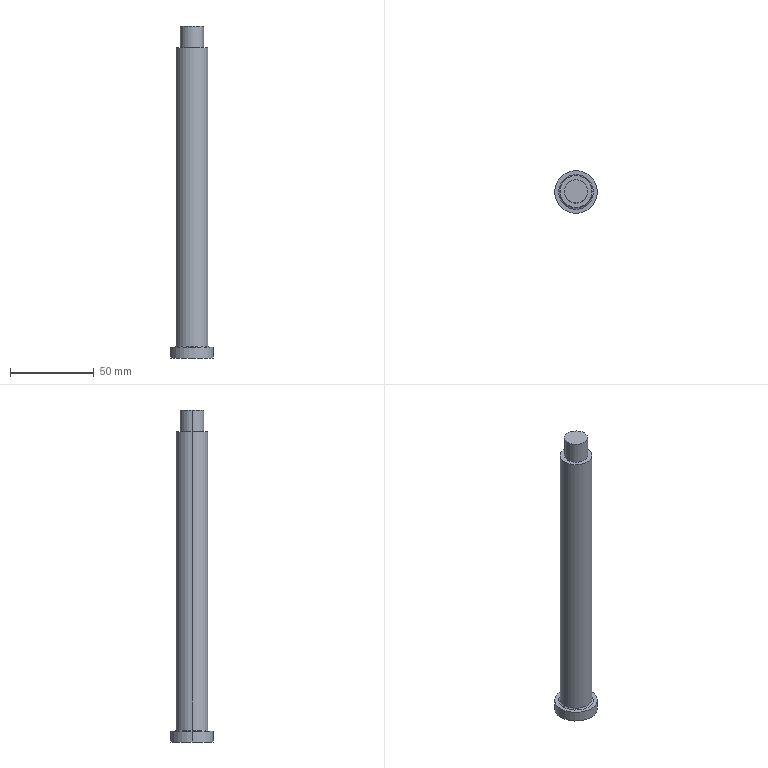Part | STEP file | 4-20.sldasm-Part-374 | 1 solid | 12 faces | box 25.4 x 25.4 x 198 mm | volume 56107 mm3 | cylinder 6 | plane 4 | torus 2 | commonest cylinder face diameters 13.862 x2 19.05 x2 25.4 x2
STEP:
#1=CARTESIAN_POINT('',(4.931,227.,93.));
#2=VERTEX_POINT('',#1);
#3=CARTESIAN_POINT('',(-8.931,227.,93.));
#4=VERTEX_POINT('',#3);
#5=CARTESIAN_POINT('',(-2.,227.,93.));
#6=DIRECTION('',(0.,0.,1.));
#7=DIRECTION('',(-1.,0.,0.));
#8=AXIS2_PLACEMENT_3D('',#5,#6,#7);
#9=CIRCLE('',#8,6.931);
#10=EDGE_CURVE('',#2,#4,#9,.T.);
#11=ORIENTED_EDGE('',*,*,#10,.F.);
#12=CARTESIAN_POINT('',(4.931,227.,80.));
#13=VERTEX_POINT('',#12);
#14=CARTESIAN_POINT('',(4.931,227.,62.4));
#15=DIRECTION('',(0.,0.,-1.));
#16=VECTOR('',#15,1000.);
#17=LINE('',#14,#16);
#18=EDGE_CURVE('',#2,#13,#17,.T.);
#19=ORIENTED_EDGE('',*,*,#18,.T.);
#20=CARTESIAN_POINT('',(-8.931,227.,80.));
#21=VERTEX_POINT('',#20);
#22=CARTESIAN_POINT('',(-2.,227.,80.));
#23=DIRECTION('',(0.,0.,1.));
#24=DIRECTION('',(1.,0.,0.));
#25=AXIS2_PLACEMENT_3D('',#22,#23,#24);
#26=CIRCLE('',#25,6.931);
#27=EDGE_CURVE('',#13,#21,#26,.T.);
#28=ORIENTED_EDGE('',*,*,#27,.T.);
#29=CARTESIAN_POINT('',(-8.931,227.,62.4));
#30=DIRECTION('',(0.,0.,-1.));
#31=VECTOR('',#30,1000.);
#32=LINE('',#29,#31);
#33=EDGE_CURVE('',#4,#21,#32,.T.);
#34=ORIENTED_EDGE('',*,*,#33,.F.);
#35=EDGE_LOOP('',(#11,#19,#28,#34));
#36=FACE_OUTER_BOUND('',#35,.T.);
#37=CARTESIAN_POINT('',(-2.,227.,62.4));
#38=DIRECTION('',(0.,0.,-1.));
#39=DIRECTION('',(-1.,0.,0.));
#40=AXIS2_PLACEMENT_3D('',#37,#38,#39);
#41=CYLINDRICAL_SURFACE('',#40,6.931);
#42=ADVANCED_FACE('',(#36),#41,.T.);
#43=CARTESIAN_POINT('',(-12.319,227.,-98.65));
#44=VERTEX_POINT('',#43);
#45=CARTESIAN_POINT('',(8.319,227.,-98.65));
#46=VERTEX_POINT('',#45);
#47=CARTESIAN_POINT('',(-2.,227.,-98.65));
#48=DIRECTION('',(0.,0.,1.));
#49=DIRECTION('',(0.,-1.,0.));
#50=AXIS2_PLACEMENT_3D('',#47,#48,#49);
#51=CIRCLE('',#50,10.319);
#52=EDGE_CURVE('',#44,#46,#51,.T.);
#53=ORIENTED_EDGE('',*,*,#52,.T.);
#54=CARTESIAN_POINT('',(7.525,227.,-97.856));
#55=VERTEX_POINT('',#54);
#56=CARTESIAN_POINT('',(8.319,227.,-97.856));
#57=DIRECTION('',(0.,1.,0.));
#58=DIRECTION('',(-1.,0.,0.));
#59=AXIS2_PLACEMENT_3D('',#56,#57,#58);
#60=CIRCLE('',#59,0.7938);
#61=EDGE_CURVE('',#46,#55,#60,.T.);
#62=ORIENTED_EDGE('',*,*,#61,.T.);
#63=CARTESIAN_POINT('',(-11.525,227.,-97.856));
#64=VERTEX_POINT('',#63);
#65=CARTESIAN_POINT('',(-2.,227.,-97.856));
#66=DIRECTION('',(0.,0.,1.));
#67=DIRECTION('',(0.,-1.,0.));
#68=AXIS2_PLACEMENT_3D('',#65,#66,#67);
#69=CIRCLE('',#68,9.525);
#70=EDGE_CURVE('',#64,#55,#69,.T.);
#71=ORIENTED_EDGE('',*,*,#70,.F.);
#72=CARTESIAN_POINT('',(-12.319,227.,-97.856));
#73=DIRECTION('',(0.,-1.,0.));
#74=DIRECTION('',(0.,0.,-1.));
#75=AXIS2_PLACEMENT_3D('',#72,#73,#74);
#76=CIRCLE('',#75,0.7937);
#77=EDGE_CURVE('',#44,#64,#76,.T.);
#78=ORIENTED_EDGE('',*,*,#77,.F.);
#79=EDGE_LOOP('',(#53,#62,#71,#78));
#80=FACE_OUTER_BOUND('',#79,.T.);
#81=CARTESIAN_POINT('',(-2.,227.,-97.856));
#82=DIRECTION('',(0.,0.,-1.));
#83=DIRECTION('',(-1.,0.,0.));
#84=AXIS2_PLACEMENT_3D('',#81,#82,#83);
#85=TOROIDAL_SURFACE('',#84,10.319,0.7937);
#86=ADVANCED_FACE('',(#80),#85,.F.);
#87=CARTESIAN_POINT('',(10.7,227.,-105.));
#88=VERTEX_POINT('',#87);
#89=CARTESIAN_POINT('',(-14.7,227.,-105.));
#90=VERTEX_POINT('',#89);
#91=CARTESIAN_POINT('',(-2.,227.,-105.));
#92=DIRECTION('',(0.,0.,1.));
#93=DIRECTION('',(0.,-1.,0.));
#94=AXIS2_PLACEMENT_3D('',#91,#92,#93);
#95=CIRCLE('',#94,12.7);
#96=EDGE_CURVE('',#88,#90,#95,.T.);
#97=ORIENTED_EDGE('',*,*,#96,.T.);
#98=CARTESIAN_POINT('',(-14.7,227.,-98.65));
#99=VERTEX_POINT('',#98);
#100=CARTESIAN_POINT('',(-14.7,227.,-101.825));
#101=DIRECTION('',(0.,0.,1.));
#102=VECTOR('',#101,1000.);
#103=LINE('',#100,#102);
#104=EDGE_CURVE('',#90,#99,#103,.T.);
#105=ORIENTED_EDGE('',*,*,#104,.T.);
#106=CARTESIAN_POINT('',(10.7,227.,-98.65));
#107=VERTEX_POINT('',#106);
#108=CARTESIAN_POINT('',(-2.,227.,-98.65));
#109=DIRECTION('',(0.,0.,1.));
#110=DIRECTION('',(0.,-1.,0.));
#111=AXIS2_PLACEMENT_3D('',#108,#109,#110);
#112=CIRCLE('',#111,12.7);
#113=EDGE_CURVE('',#107,#99,#112,.T.);
#114=ORIENTED_EDGE('',*,*,#113,.F.);
#115=CARTESIAN_POINT('',(10.7,227.,-101.825));
#116=DIRECTION('',(0.,0.,1.));
#117=VECTOR('',#116,1000.);
#118=LINE('',#115,#117);
#119=EDGE_CURVE('',#88,#107,#118,.T.);
#120=ORIENTED_EDGE('',*,*,#119,.F.);
#121=EDGE_LOOP('',(#97,#105,#114,#120));
#122=FACE_OUTER_BOUND('',#121,.T.);
#123=CARTESIAN_POINT('',(-2.,227.,-101.825));
#124=DIRECTION('',(0.,0.,1.));
#125=DIRECTION('',(1.,0.,0.));
#126=AXIS2_PLACEMENT_3D('',#123,#124,#125);
#127=CYLINDRICAL_SURFACE('',#126,12.7);
#128=ADVANCED_FACE('',(#122),#127,.T.);
#129=CARTESIAN_POINT('',(-2.,227.,-97.856));
#130=DIRECTION('',(0.,0.,1.));
#131=DIRECTION('',(0.,-1.,0.));
#132=AXIS2_PLACEMENT_3D('',#129,#130,#131);
#133=CIRCLE('',#132,9.525);
#134=EDGE_CURVE('',#55,#64,#133,.T.);
#135=ORIENTED_EDGE('',*,*,#134,.T.);
#136=CARTESIAN_POINT('',(-11.525,227.,80.));
#137=VERTEX_POINT('',#136);
#138=CARTESIAN_POINT('',(-11.525,227.,-25.228));
#139=DIRECTION('',(0.,0.,1.));
#140=VECTOR('',#139,1000.);
#141=LINE('',#138,#140);
#142=EDGE_CURVE('',#64,#137,#141,.T.);
#143=ORIENTED_EDGE('',*,*,#142,.T.);
#144=CARTESIAN_POINT('',(7.525,227.,80.));
#145=VERTEX_POINT('',#144);
#146=CARTESIAN_POINT('',(-2.,227.,80.));
#147=DIRECTION('',(0.,0.,1.));
#148=DIRECTION('',(1.,0.,0.));
#149=AXIS2_PLACEMENT_3D('',#146,#147,#148);
#150=CIRCLE('',#149,9.525);
#151=EDGE_CURVE('',#145,#137,#150,.T.);
#152=ORIENTED_EDGE('',*,*,#151,.F.);
#153=CARTESIAN_POINT('',(7.525,227.,-25.228));
#154=DIRECTION('',(0.,0.,1.));
#155=VECTOR('',#154,1000.);
#156=LINE('',#153,#155);
#157=EDGE_CURVE('',#55,#145,#156,.T.);
#158=ORIENTED_EDGE('',*,*,#157,.F.);
#159=EDGE_LOOP('',(#135,#143,#152,#158));
#160=FACE_OUTER_BOUND('',#159,.T.);
#161=CARTESIAN_POINT('',(-2.,227.,-25.228));
#162=DIRECTION('',(0.,0.,1.));
#163=DIRECTION('',(1.,0.,0.));
#164=AXIS2_PLACEMENT_3D('',#161,#162,#163);
#165=CYLINDRICAL_SURFACE('',#164,9.525);
#166=ADVANCED_FACE('',(#160),#165,.T.);
#167=ORIENTED_EDGE('',*,*,#151,.T.);
#168=CARTESIAN_POINT('',(-2.,227.,80.));
#169=DIRECTION('',(0.,0.,1.));
#170=DIRECTION('',(1.,0.,0.));
#171=AXIS2_PLACEMENT_3D('',#168,#169,#170);
#172=CIRCLE('',#171,9.525);
#173=EDGE_CURVE('',#137,#145,#172,.T.);
#174=ORIENTED_EDGE('',*,*,#173,.T.);
#175=EDGE_LOOP('',(#167,#174));
#176=FACE_OUTER_BOUND('',#175,.T.);
#177=CARTESIAN_POINT('',(-2.,227.,80.));
#178=DIRECTION('',(0.,0.,1.));
#179=DIRECTION('',(1.,0.,0.));
#180=AXIS2_PLACEMENT_3D('',#177,#178,#179);
#181=CIRCLE('',#180,6.931);
#182=EDGE_CURVE('',#21,#13,#181,.T.);
#183=ORIENTED_EDGE('',*,*,#182,.F.);
#184=ORIENTED_EDGE('',*,*,#27,.F.);
#185=EDGE_LOOP('',(#183,#184));
#186=FACE_BOUND('',#185,.T.);
#187=CARTESIAN_POINT('',(-2.,227.,80.));
#188=DIRECTION('',(0.,0.,1.));
#189=DIRECTION('',(1.,0.,0.));
#190=AXIS2_PLACEMENT_3D('',#187,#188,#189);
#191=PLANE('',#190);
#192=ADVANCED_FACE('',(#176,#186),#191,.T.);
#193=ORIENTED_EDGE('',*,*,#142,.F.);
#194=ORIENTED_EDGE('',*,*,#70,.T.);
#195=ORIENTED_EDGE('',*,*,#157,.T.);
#196=ORIENTED_EDGE('',*,*,#173,.F.);
#197=EDGE_LOOP('',(#193,#194,#195,#196));
#198=FACE_OUTER_BOUND('',#197,.T.);
#199=CARTESIAN_POINT('',(-2.,227.,-25.228));
#200=DIRECTION('',(0.,0.,1.));
#201=DIRECTION('',(1.,0.,0.));
#202=AXIS2_PLACEMENT_3D('',#199,#200,#201);
#203=CYLINDRICAL_SURFACE('',#202,9.525);
#204=ADVANCED_FACE('',(#198),#203,.T.);
#205=ORIENTED_EDGE('',*,*,#96,.F.);
#206=CARTESIAN_POINT('',(-2.,227.,-105.));
#207=DIRECTION('',(0.,0.,1.));
#208=DIRECTION('',(0.,-1.,0.));
#209=AXIS2_PLACEMENT_3D('',#206,#207,#208);
#210=CIRCLE('',#209,12.7);
#211=EDGE_CURVE('',#90,#88,#210,.T.);
#212=ORIENTED_EDGE('',*,*,#211,.F.);
#213=EDGE_LOOP('',(#205,#212));
#214=FACE_OUTER_BOUND('',#213,.T.);
#215=CARTESIAN_POINT('',(-2.,220.65,-105.));
#216=DIRECTION('',(0.,0.,-1.));
#217=DIRECTION('',(-1.,0.,0.));
#218=AXIS2_PLACEMENT_3D('',#215,#216,#217);
#219=PLANE('',#218);
#220=ADVANCED_FACE('',(#214),#219,.T.);
#221=ORIENTED_EDGE('',*,*,#104,.F.);
#222=ORIENTED_EDGE('',*,*,#211,.T.);
#223=ORIENTED_EDGE('',*,*,#119,.T.);
#224=CARTESIAN_POINT('',(-2.,227.,-98.65));
#225=DIRECTION('',(0.,0.,1.));
#226=DIRECTION('',(0.,-1.,0.));
#227=AXIS2_PLACEMENT_3D('',#224,#225,#226);
#228=CIRCLE('',#227,12.7);
#229=EDGE_CURVE('',#99,#107,#228,.T.);
#230=ORIENTED_EDGE('',*,*,#229,.F.);
#231=EDGE_LOOP('',(#221,#222,#223,#230));
#232=FACE_OUTER_BOUND('',#231,.T.);
#233=CARTESIAN_POINT('',(-2.,227.,-101.825));
#234=DIRECTION('',(0.,0.,1.));
#235=DIRECTION('',(1.,0.,0.));
#236=AXIS2_PLACEMENT_3D('',#233,#234,#235);
#237=CYLINDRICAL_SURFACE('',#236,12.7);
#238=ADVANCED_FACE('',(#232),#237,.T.);
#239=ORIENTED_EDGE('',*,*,#61,.F.);
#240=CARTESIAN_POINT('',(-2.,227.,-98.65));
#241=DIRECTION('',(0.,0.,1.));
#242=DIRECTION('',(0.,-1.,0.));
#243=AXIS2_PLACEMENT_3D('',#240,#241,#242);
#244=CIRCLE('',#243,10.319);
#245=EDGE_CURVE('',#46,#44,#244,.T.);
#246=ORIENTED_EDGE('',*,*,#245,.T.);
#247=ORIENTED_EDGE('',*,*,#77,.T.);
#248=ORIENTED_EDGE('',*,*,#134,.F.);
#249=EDGE_LOOP('',(#239,#246,#247,#248));
#250=FACE_OUTER_BOUND('',#249,.T.);
#251=CARTESIAN_POINT('',(-2.,227.,-97.856));
#252=DIRECTION('',(0.,0.,-1.));
#253=DIRECTION('',(-1.,0.,0.));
#254=AXIS2_PLACEMENT_3D('',#251,#252,#253);
#255=TOROIDAL_SURFACE('',#254,10.319,0.7937);
#256=ADVANCED_FACE('',(#250),#255,.F.);
#257=ORIENTED_EDGE('',*,*,#113,.T.);
#258=ORIENTED_EDGE('',*,*,#229,.T.);
#259=EDGE_LOOP('',(#257,#258));
#260=FACE_OUTER_BOUND('',#259,.T.);
#261=ORIENTED_EDGE('',*,*,#52,.F.);
#262=ORIENTED_EDGE('',*,*,#245,.F.);
#263=EDGE_LOOP('',(#261,#262));
#264=FACE_BOUND('',#263,.T.);
#265=CARTESIAN_POINT('',(-2.,215.491,-98.65));
#266=DIRECTION('',(0.,0.,1.));
#267=DIRECTION('',(1.,0.,0.));
#268=AXIS2_PLACEMENT_3D('',#265,#266,#267);
#269=PLANE('',#268);
#270=ADVANCED_FACE('',(#260,#264),#269,.T.);
#271=ORIENTED_EDGE('',*,*,#18,.F.);
#272=CARTESIAN_POINT('',(-2.,227.,93.));
#273=DIRECTION('',(0.,0.,1.));
#274=DIRECTION('',(-1.,0.,0.));
#275=AXIS2_PLACEMENT_3D('',#272,#273,#274);
#276=CIRCLE('',#275,6.931);
#277=EDGE_CURVE('',#4,#2,#276,.T.);
#278=ORIENTED_EDGE('',*,*,#277,.F.);
#279=ORIENTED_EDGE('',*,*,#33,.T.);
#280=ORIENTED_EDGE('',*,*,#182,.T.);
#281=EDGE_LOOP('',(#271,#278,#279,#280));
#282=FACE_OUTER_BOUND('',#281,.T.);
#283=CARTESIAN_POINT('',(-2.,227.,62.4));
#284=DIRECTION('',(0.,0.,-1.));
#285=DIRECTION('',(-1.,0.,0.));
#286=AXIS2_PLACEMENT_3D('',#283,#284,#285);
#287=CYLINDRICAL_SURFACE('',#286,6.931);
#288=ADVANCED_FACE('',(#282),#287,.T.);
#289=ORIENTED_EDGE('',*,*,#277,.T.);
#290=ORIENTED_EDGE('',*,*,#10,.T.);
#291=EDGE_LOOP('',(#289,#290));
#292=FACE_OUTER_BOUND('',#291,.T.);
#293=CARTESIAN_POINT('',(-2.,-93.,93.));
#294=DIRECTION('',(0.,0.,-1.));
#295=DIRECTION('',(-1.,0.,0.));
#296=AXIS2_PLACEMENT_3D('',#293,#294,#295);
#297=PLANE('',#296);
#298=ADVANCED_FACE('',(#292),#297,.F.);
#299=CLOSED_SHELL('',(#42,#86,#128,#166,#192,#204,#220,#238,#256,#270,#288,#298));
#300=MANIFOLD_SOLID_BREP('',#299);
#301=CARTESIAN_POINT('',(0.,0.,0.));
#302=DIRECTION('',(0.,0.,1.));
#303=DIRECTION('',(1.,0.,0.));
#304=AXIS2_PLACEMENT_3D('',#301,#302,#303);
#305=(LENGTH_UNIT()NAMED_UNIT(*)SI_UNIT(.MILLI.,.METRE.));
#306=UNCERTAINTY_MEASURE_WITH_UNIT(LENGTH_MEASURE(0.00001),#305,'','');
#307=(NAMED_UNIT(*)PLANE_ANGLE_UNIT()SI_UNIT($,.RADIAN.));
#308=(NAMED_UNIT(*)SI_UNIT($,.STERADIAN.)SOLID_ANGLE_UNIT());
#309=(GEOMETRIC_REPRESENTATION_CONTEXT(3)GLOBAL_UNCERTAINTY_ASSIGNED_CONTEXT((#306))GLOBAL_UNIT_ASSIGNED_CONTEXT((#305,#307,#308))REPRESENTATION_CONTEXT('',''));
#310=ADVANCED_BREP_SHAPE_REPRESENTATION('',(#300,#304),#309);